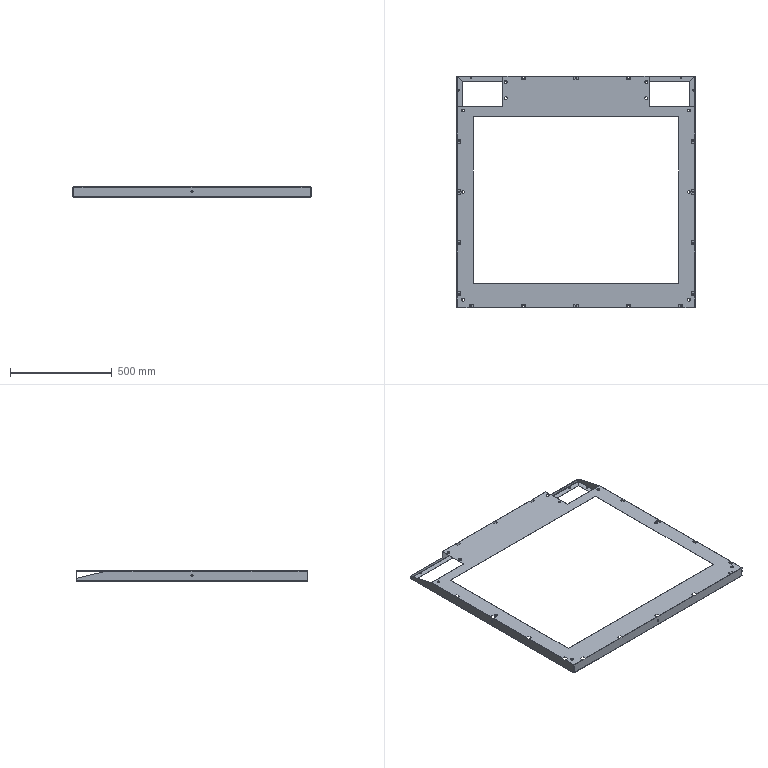Part | 1 solid | 360 faces | box 1169 x 1139 x 50 mm | volume 748825 mm3 | plane 224 | cylinder 124 | spline 12 | commonest cylinder face diameters 7 x50 0.4 x24 2.4 x24 14 x20 10 x6